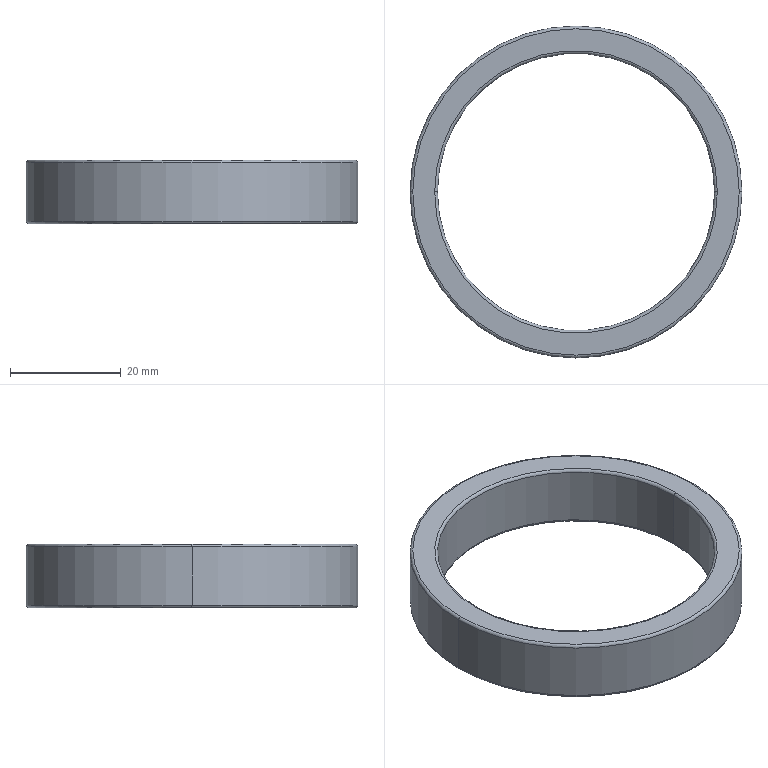Part | STEP file | 10-06 shaft shoulder | 1 solid | 14 faces | box 60 x 60 x 11.5 mm | volume 9808 mm3 | torus 8 | cylinder 4 | plane 2 | commonest cylinder face diameters 50.1 x2 60 x2
STEP:
#1=CARTESIAN_POINT('',(-30.,0.,5.25));
#2=VERTEX_POINT('',#1);
#3=CARTESIAN_POINT('',(30.,0.,5.25));
#4=VERTEX_POINT('',#3);
#5=CARTESIAN_POINT('',(0.,0.,5.25));
#6=DIRECTION('',(0.,0.,-1.));
#7=DIRECTION('',(1.,0.,0.));
#8=AXIS2_PLACEMENT_3D('',#5,#6,#7);
#9=CIRCLE('',#8,30.);
#10=EDGE_CURVE('',#2,#4,#9,.T.);
#11=ORIENTED_EDGE('',*,*,#10,.F.);
#12=CARTESIAN_POINT('',(-29.5,0.,5.75));
#13=VERTEX_POINT('',#12);
#14=CARTESIAN_POINT('',(-29.5,0.,5.25));
#15=DIRECTION('',(0.,1.,0.));
#16=DIRECTION('',(-1.,0.,0.));
#17=AXIS2_PLACEMENT_3D('',#14,#15,#16);
#18=CIRCLE('',#17,0.5);
#19=EDGE_CURVE('',#2,#13,#18,.T.);
#20=ORIENTED_EDGE('',*,*,#19,.T.);
#21=CARTESIAN_POINT('',(29.5,0.,5.75));
#22=VERTEX_POINT('',#21);
#23=CARTESIAN_POINT('',(0.,0.,5.75));
#24=DIRECTION('',(0.,0.,1.));
#25=DIRECTION('',(1.,0.,0.));
#26=AXIS2_PLACEMENT_3D('',#23,#24,#25);
#27=CIRCLE('',#26,29.5);
#28=EDGE_CURVE('',#22,#13,#27,.T.);
#29=ORIENTED_EDGE('',*,*,#28,.F.);
#30=CARTESIAN_POINT('',(29.5,0.,5.25));
#31=DIRECTION('',(0.,-1.,0.));
#32=DIRECTION('',(0.,0.,-1.));
#33=AXIS2_PLACEMENT_3D('',#30,#31,#32);
#34=CIRCLE('',#33,0.5);
#35=EDGE_CURVE('',#4,#22,#34,.T.);
#36=ORIENTED_EDGE('',*,*,#35,.F.);
#37=EDGE_LOOP('',(#11,#20,#29,#36));
#38=FACE_OUTER_BOUND('',#37,.T.);
#39=CARTESIAN_POINT('',(0.,0.,5.25));
#40=DIRECTION('',(0.,0.,1.));
#41=DIRECTION('',(1.,0.,0.));
#42=AXIS2_PLACEMENT_3D('',#39,#40,#41);
#43=TOROIDAL_SURFACE('',#42,29.5,0.5);
#44=ADVANCED_FACE('',(#38),#43,.T.);
#45=CARTESIAN_POINT('',(-29.5,0.,-5.75));
#46=VERTEX_POINT('',#45);
#47=CARTESIAN_POINT('',(29.5,0.,-5.75));
#48=VERTEX_POINT('',#47);
#49=CARTESIAN_POINT('',(0.,0.,-5.75));
#50=DIRECTION('',(0.,0.,-1.));
#51=DIRECTION('',(1.,0.,0.));
#52=AXIS2_PLACEMENT_3D('',#49,#50,#51);
#53=CIRCLE('',#52,29.5);
#54=EDGE_CURVE('',#46,#48,#53,.T.);
#55=ORIENTED_EDGE('',*,*,#54,.F.);
#56=CARTESIAN_POINT('',(-30.,0.,-5.25));
#57=VERTEX_POINT('',#56);
#58=CARTESIAN_POINT('',(-29.5,0.,-5.25));
#59=DIRECTION('',(0.,1.,0.));
#60=DIRECTION('',(-1.,0.,0.));
#61=AXIS2_PLACEMENT_3D('',#58,#59,#60);
#62=CIRCLE('',#61,0.5);
#63=EDGE_CURVE('',#46,#57,#62,.T.);
#64=ORIENTED_EDGE('',*,*,#63,.T.);
#65=CARTESIAN_POINT('',(30.,0.,-5.25));
#66=VERTEX_POINT('',#65);
#67=CARTESIAN_POINT('',(0.,0.,-5.25));
#68=DIRECTION('',(0.,0.,1.));
#69=DIRECTION('',(1.,0.,0.));
#70=AXIS2_PLACEMENT_3D('',#67,#68,#69);
#71=CIRCLE('',#70,30.);
#72=EDGE_CURVE('',#66,#57,#71,.T.);
#73=ORIENTED_EDGE('',*,*,#72,.F.);
#74=CARTESIAN_POINT('',(29.5,0.,-5.25));
#75=DIRECTION('',(0.,-1.,0.));
#76=DIRECTION('',(0.,0.,-1.));
#77=AXIS2_PLACEMENT_3D('',#74,#75,#76);
#78=CIRCLE('',#77,0.5);
#79=EDGE_CURVE('',#48,#66,#78,.T.);
#80=ORIENTED_EDGE('',*,*,#79,.F.);
#81=EDGE_LOOP('',(#55,#64,#73,#80));
#82=FACE_OUTER_BOUND('',#81,.T.);
#83=CARTESIAN_POINT('',(0.,0.,-5.25));
#84=DIRECTION('',(0.,0.,1.));
#85=DIRECTION('',(1.,0.,0.));
#86=AXIS2_PLACEMENT_3D('',#83,#84,#85);
#87=TOROIDAL_SURFACE('',#86,29.5,0.5);
#88=ADVANCED_FACE('',(#82),#87,.T.);
#89=CARTESIAN_POINT('',(-25.05,0.,-5.25));
#90=VERTEX_POINT('',#89);
#91=CARTESIAN_POINT('',(25.05,0.,-5.25));
#92=VERTEX_POINT('',#91);
#93=CARTESIAN_POINT('',(0.,0.,-5.25));
#94=DIRECTION('',(0.,0.,-1.));
#95=DIRECTION('',(1.,0.,0.));
#96=AXIS2_PLACEMENT_3D('',#93,#94,#95);
#97=CIRCLE('',#96,25.05);
#98=EDGE_CURVE('',#90,#92,#97,.T.);
#99=ORIENTED_EDGE('',*,*,#98,.F.);
#100=CARTESIAN_POINT('',(-25.55,0.,-5.75));
#101=VERTEX_POINT('',#100);
#102=CARTESIAN_POINT('',(-25.55,0.,-5.25));
#103=DIRECTION('',(0.,1.,0.));
#104=DIRECTION('',(-1.,0.,0.));
#105=AXIS2_PLACEMENT_3D('',#102,#103,#104);
#106=CIRCLE('',#105,0.5);
#107=EDGE_CURVE('',#90,#101,#106,.T.);
#108=ORIENTED_EDGE('',*,*,#107,.T.);
#109=CARTESIAN_POINT('',(25.55,0.,-5.75));
#110=VERTEX_POINT('',#109);
#111=CARTESIAN_POINT('',(0.,0.,-5.75));
#112=DIRECTION('',(0.,0.,1.));
#113=DIRECTION('',(1.,0.,0.));
#114=AXIS2_PLACEMENT_3D('',#111,#112,#113);
#115=CIRCLE('',#114,25.55);
#116=EDGE_CURVE('',#110,#101,#115,.T.);
#117=ORIENTED_EDGE('',*,*,#116,.F.);
#118=CARTESIAN_POINT('',(25.55,0.,-5.25));
#119=DIRECTION('',(0.,-1.,0.));
#120=DIRECTION('',(0.,0.,-1.));
#121=AXIS2_PLACEMENT_3D('',#118,#119,#120);
#122=CIRCLE('',#121,0.5);
#123=EDGE_CURVE('',#92,#110,#122,.T.);
#124=ORIENTED_EDGE('',*,*,#123,.F.);
#125=EDGE_LOOP('',(#99,#108,#117,#124));
#126=FACE_OUTER_BOUND('',#125,.T.);
#127=CARTESIAN_POINT('',(0.,0.,-5.25));
#128=DIRECTION('',(0.,0.,1.));
#129=DIRECTION('',(1.,0.,0.));
#130=AXIS2_PLACEMENT_3D('',#127,#128,#129);
#131=TOROIDAL_SURFACE('',#130,25.55,0.5);
#132=ADVANCED_FACE('',(#126),#131,.T.);
#133=CARTESIAN_POINT('',(-25.55,0.,5.75));
#134=VERTEX_POINT('',#133);
#135=CARTESIAN_POINT('',(25.55,0.,5.75));
#136=VERTEX_POINT('',#135);
#137=CARTESIAN_POINT('',(0.,0.,5.75));
#138=DIRECTION('',(0.,0.,-1.));
#139=DIRECTION('',(1.,0.,0.));
#140=AXIS2_PLACEMENT_3D('',#137,#138,#139);
#141=CIRCLE('',#140,25.55);
#142=EDGE_CURVE('',#134,#136,#141,.T.);
#143=ORIENTED_EDGE('',*,*,#142,.F.);
#144=CARTESIAN_POINT('',(-25.05,0.,5.25));
#145=VERTEX_POINT('',#144);
#146=CARTESIAN_POINT('',(-25.55,0.,5.25));
#147=DIRECTION('',(0.,1.,0.));
#148=DIRECTION('',(-1.,0.,0.));
#149=AXIS2_PLACEMENT_3D('',#146,#147,#148);
#150=CIRCLE('',#149,0.5);
#151=EDGE_CURVE('',#134,#145,#150,.T.);
#152=ORIENTED_EDGE('',*,*,#151,.T.);
#153=CARTESIAN_POINT('',(25.05,0.,5.25));
#154=VERTEX_POINT('',#153);
#155=CARTESIAN_POINT('',(0.,0.,5.25));
#156=DIRECTION('',(0.,0.,1.));
#157=DIRECTION('',(1.,0.,0.));
#158=AXIS2_PLACEMENT_3D('',#155,#156,#157);
#159=CIRCLE('',#158,25.05);
#160=EDGE_CURVE('',#154,#145,#159,.T.);
#161=ORIENTED_EDGE('',*,*,#160,.F.);
#162=CARTESIAN_POINT('',(25.55,0.,5.25));
#163=DIRECTION('',(0.,-1.,0.));
#164=DIRECTION('',(0.,0.,-1.));
#165=AXIS2_PLACEMENT_3D('',#162,#163,#164);
#166=CIRCLE('',#165,0.5);
#167=EDGE_CURVE('',#136,#154,#166,.T.);
#168=ORIENTED_EDGE('',*,*,#167,.F.);
#169=EDGE_LOOP('',(#143,#152,#161,#168));
#170=FACE_OUTER_BOUND('',#169,.T.);
#171=CARTESIAN_POINT('',(0.,0.,5.25));
#172=DIRECTION('',(0.,0.,1.));
#173=DIRECTION('',(1.,0.,0.));
#174=AXIS2_PLACEMENT_3D('',#171,#172,#173);
#175=TOROIDAL_SURFACE('',#174,25.55,0.5);
#176=ADVANCED_FACE('',(#170),#175,.T.);
#177=CARTESIAN_POINT('',(0.,0.,5.25));
#178=DIRECTION('',(0.,0.,1.));
#179=DIRECTION('',(1.,0.,0.));
#180=AXIS2_PLACEMENT_3D('',#177,#178,#179);
#181=CIRCLE('',#180,25.05);
#182=EDGE_CURVE('',#145,#154,#181,.T.);
#183=ORIENTED_EDGE('',*,*,#182,.T.);
#184=CARTESIAN_POINT('',(25.05,0.,5.75));
#185=DIRECTION('',(0.,0.,-1.));
#186=VECTOR('',#185,1000.);
#187=LINE('',#184,#186);
#188=EDGE_CURVE('',#154,#92,#187,.T.);
#189=ORIENTED_EDGE('',*,*,#188,.T.);
#190=CARTESIAN_POINT('',(0.,0.,-5.25));
#191=DIRECTION('',(0.,0.,-1.));
#192=DIRECTION('',(1.,0.,0.));
#193=AXIS2_PLACEMENT_3D('',#190,#191,#192);
#194=CIRCLE('',#193,25.05);
#195=EDGE_CURVE('',#92,#90,#194,.T.);
#196=ORIENTED_EDGE('',*,*,#195,.T.);
#197=CARTESIAN_POINT('',(-25.05,0.,5.75));
#198=DIRECTION('',(0.,0.,-1.));
#199=VECTOR('',#198,1000.);
#200=LINE('',#197,#199);
#201=EDGE_CURVE('',#145,#90,#200,.T.);
#202=ORIENTED_EDGE('',*,*,#201,.F.);
#203=EDGE_LOOP('',(#183,#189,#196,#202));
#204=FACE_OUTER_BOUND('',#203,.T.);
#205=CARTESIAN_POINT('',(0.,0.,5.75));
#206=DIRECTION('',(0.,0.,-1.));
#207=DIRECTION('',(-1.,0.,0.));
#208=AXIS2_PLACEMENT_3D('',#205,#206,#207);
#209=CYLINDRICAL_SURFACE('',#208,25.05);
#210=ADVANCED_FACE('',(#204),#209,.F.);
#211=ORIENTED_EDGE('',*,*,#10,.T.);
#212=CARTESIAN_POINT('',(30.,0.,5.75));
#213=DIRECTION('',(0.,0.,-1.));
#214=VECTOR('',#213,1000.);
#215=LINE('',#212,#214);
#216=EDGE_CURVE('',#4,#66,#215,.T.);
#217=ORIENTED_EDGE('',*,*,#216,.T.);
#218=ORIENTED_EDGE('',*,*,#72,.T.);
#219=CARTESIAN_POINT('',(-30.,0.,5.75));
#220=DIRECTION('',(0.,0.,-1.));
#221=VECTOR('',#220,1000.);
#222=LINE('',#219,#221);
#223=EDGE_CURVE('',#2,#57,#222,.T.);
#224=ORIENTED_EDGE('',*,*,#223,.F.);
#225=EDGE_LOOP('',(#211,#217,#218,#224));
#226=FACE_OUTER_BOUND('',#225,.T.);
#227=CARTESIAN_POINT('',(0.,0.,5.75));
#228=DIRECTION('',(0.,0.,-1.));
#229=DIRECTION('',(-1.,0.,0.));
#230=AXIS2_PLACEMENT_3D('',#227,#228,#229);
#231=CYLINDRICAL_SURFACE('',#230,30.);
#232=ADVANCED_FACE('',(#226),#231,.T.);
#233=CARTESIAN_POINT('',(0.,0.,5.75));
#234=DIRECTION('',(0.,0.,-1.));
#235=DIRECTION('',(1.,0.,0.));
#236=AXIS2_PLACEMENT_3D('',#233,#234,#235);
#237=CIRCLE('',#236,25.55);
#238=EDGE_CURVE('',#136,#134,#237,.T.);
#239=ORIENTED_EDGE('',*,*,#238,.T.);
#240=ORIENTED_EDGE('',*,*,#142,.T.);
#241=EDGE_LOOP('',(#239,#240));
#242=FACE_BOUND('',#241,.T.);
#243=ORIENTED_EDGE('',*,*,#28,.T.);
#244=CARTESIAN_POINT('',(0.,0.,5.75));
#245=DIRECTION('',(0.,0.,1.));
#246=DIRECTION('',(1.,0.,0.));
#247=AXIS2_PLACEMENT_3D('',#244,#245,#246);
#248=CIRCLE('',#247,29.5);
#249=EDGE_CURVE('',#13,#22,#248,.T.);
#250=ORIENTED_EDGE('',*,*,#249,.T.);
#251=EDGE_LOOP('',(#243,#250));
#252=FACE_OUTER_BOUND('',#251,.T.);
#253=CARTESIAN_POINT('',(0.,0.,5.75));
#254=DIRECTION('',(0.,0.,1.));
#255=DIRECTION('',(1.,0.,0.));
#256=AXIS2_PLACEMENT_3D('',#253,#254,#255);
#257=PLANE('',#256);
#258=ADVANCED_FACE('',(#242,#252),#257,.T.);
#259=ORIENTED_EDGE('',*,*,#116,.T.);
#260=CARTESIAN_POINT('',(0.,0.,-5.75));
#261=DIRECTION('',(0.,0.,1.));
#262=DIRECTION('',(1.,0.,0.));
#263=AXIS2_PLACEMENT_3D('',#260,#261,#262);
#264=CIRCLE('',#263,25.55);
#265=EDGE_CURVE('',#101,#110,#264,.T.);
#266=ORIENTED_EDGE('',*,*,#265,.T.);
#267=EDGE_LOOP('',(#259,#266));
#268=FACE_BOUND('',#267,.T.);
#269=CARTESIAN_POINT('',(0.,0.,-5.75));
#270=DIRECTION('',(0.,0.,-1.));
#271=DIRECTION('',(1.,0.,0.));
#272=AXIS2_PLACEMENT_3D('',#269,#270,#271);
#273=CIRCLE('',#272,29.5);
#274=EDGE_CURVE('',#48,#46,#273,.T.);
#275=ORIENTED_EDGE('',*,*,#274,.T.);
#276=ORIENTED_EDGE('',*,*,#54,.T.);
#277=EDGE_LOOP('',(#275,#276));
#278=FACE_OUTER_BOUND('',#277,.T.);
#279=CARTESIAN_POINT('',(0.,0.,-5.75));
#280=DIRECTION('',(0.,0.,1.));
#281=DIRECTION('',(1.,0.,0.));
#282=AXIS2_PLACEMENT_3D('',#279,#280,#281);
#283=PLANE('',#282);
#284=ADVANCED_FACE('',(#268,#278),#283,.F.);
#285=ORIENTED_EDGE('',*,*,#216,.F.);
#286=CARTESIAN_POINT('',(0.,0.,5.25));
#287=DIRECTION('',(0.,0.,-1.));
#288=DIRECTION('',(1.,0.,0.));
#289=AXIS2_PLACEMENT_3D('',#286,#287,#288);
#290=CIRCLE('',#289,30.);
#291=EDGE_CURVE('',#4,#2,#290,.T.);
#292=ORIENTED_EDGE('',*,*,#291,.T.);
#293=ORIENTED_EDGE('',*,*,#223,.T.);
#294=CARTESIAN_POINT('',(0.,0.,-5.25));
#295=DIRECTION('',(0.,0.,1.));
#296=DIRECTION('',(1.,0.,0.));
#297=AXIS2_PLACEMENT_3D('',#294,#295,#296);
#298=CIRCLE('',#297,30.);
#299=EDGE_CURVE('',#57,#66,#298,.T.);
#300=ORIENTED_EDGE('',*,*,#299,.T.);
#301=EDGE_LOOP('',(#285,#292,#293,#300));
#302=FACE_OUTER_BOUND('',#301,.T.);
#303=CARTESIAN_POINT('',(0.,0.,5.75));
#304=DIRECTION('',(0.,0.,-1.));
#305=DIRECTION('',(-1.,0.,0.));
#306=AXIS2_PLACEMENT_3D('',#303,#304,#305);
#307=CYLINDRICAL_SURFACE('',#306,30.);
#308=ADVANCED_FACE('',(#302),#307,.T.);
#309=ORIENTED_EDGE('',*,*,#188,.F.);
#310=ORIENTED_EDGE('',*,*,#160,.T.);
#311=ORIENTED_EDGE('',*,*,#201,.T.);
#312=ORIENTED_EDGE('',*,*,#98,.T.);
#313=EDGE_LOOP('',(#309,#310,#311,#312));
#314=FACE_OUTER_BOUND('',#313,.T.);
#315=CARTESIAN_POINT('',(0.,0.,5.75));
#316=DIRECTION('',(0.,0.,-1.));
#317=DIRECTION('',(-1.,0.,0.));
#318=AXIS2_PLACEMENT_3D('',#315,#316,#317);
#319=CYLINDRICAL_SURFACE('',#318,25.05);
#320=ADVANCED_FACE('',(#314),#319,.F.);
#321=ORIENTED_EDGE('',*,*,#151,.F.);
#322=ORIENTED_EDGE('',*,*,#238,.F.);
#323=ORIENTED_EDGE('',*,*,#167,.T.);
#324=ORIENTED_EDGE('',*,*,#182,.F.);
#325=EDGE_LOOP('',(#321,#322,#323,#324));
#326=FACE_OUTER_BOUND('',#325,.T.);
#327=CARTESIAN_POINT('',(0.,0.,5.25));
#328=DIRECTION('',(0.,0.,1.));
#329=DIRECTION('',(1.,0.,0.));
#330=AXIS2_PLACEMENT_3D('',#327,#328,#329);
#331=TOROIDAL_SURFACE('',#330,25.55,0.5);
#332=ADVANCED_FACE('',(#326),#331,.T.);
#333=ORIENTED_EDGE('',*,*,#107,.F.);
#334=ORIENTED_EDGE('',*,*,#195,.F.);
#335=ORIENTED_EDGE('',*,*,#123,.T.);
#336=ORIENTED_EDGE('',*,*,#265,.F.);
#337=EDGE_LOOP('',(#333,#334,#335,#336));
#338=FACE_OUTER_BOUND('',#337,.T.);
#339=CARTESIAN_POINT('',(0.,0.,-5.25));
#340=DIRECTION('',(0.,0.,1.));
#341=DIRECTION('',(1.,0.,0.));
#342=AXIS2_PLACEMENT_3D('',#339,#340,#341);
#343=TOROIDAL_SURFACE('',#342,25.55,0.5);
#344=ADVANCED_FACE('',(#338),#343,.T.);
#345=ORIENTED_EDGE('',*,*,#63,.F.);
#346=ORIENTED_EDGE('',*,*,#274,.F.);
#347=ORIENTED_EDGE('',*,*,#79,.T.);
#348=ORIENTED_EDGE('',*,*,#299,.F.);
#349=EDGE_LOOP('',(#345,#346,#347,#348));
#350=FACE_OUTER_BOUND('',#349,.T.);
#351=CARTESIAN_POINT('',(0.,0.,-5.25));
#352=DIRECTION('',(0.,0.,1.));
#353=DIRECTION('',(1.,0.,0.));
#354=AXIS2_PLACEMENT_3D('',#351,#352,#353);
#355=TOROIDAL_SURFACE('',#354,29.5,0.5);
#356=ADVANCED_FACE('',(#350),#355,.T.);
#357=ORIENTED_EDGE('',*,*,#19,.F.);
#358=ORIENTED_EDGE('',*,*,#291,.F.);
#359=ORIENTED_EDGE('',*,*,#35,.T.);
#360=ORIENTED_EDGE('',*,*,#249,.F.);
#361=EDGE_LOOP('',(#357,#358,#359,#360));
#362=FACE_OUTER_BOUND('',#361,.T.);
#363=CARTESIAN_POINT('',(0.,0.,5.25));
#364=DIRECTION('',(0.,0.,1.));
#365=DIRECTION('',(1.,0.,0.));
#366=AXIS2_PLACEMENT_3D('',#363,#364,#365);
#367=TOROIDAL_SURFACE('',#366,29.5,0.5);
#368=ADVANCED_FACE('',(#362),#367,.T.);
#369=CLOSED_SHELL('',(#44,#88,#132,#176,#210,#232,#258,#284,#308,#320,#332,#344,#356,#368));
#370=MANIFOLD_SOLID_BREP('',#369);
#371=CARTESIAN_POINT('',(0.,0.,0.));
#372=DIRECTION('',(0.,0.,1.));
#373=DIRECTION('',(1.,0.,0.));
#374=AXIS2_PLACEMENT_3D('',#371,#372,#373);
#375=(LENGTH_UNIT()NAMED_UNIT(*)SI_UNIT(.MILLI.,.METRE.));
#376=UNCERTAINTY_MEASURE_WITH_UNIT(LENGTH_MEASURE(0.00001),#375,'','');
#377=(NAMED_UNIT(*)PLANE_ANGLE_UNIT()SI_UNIT($,.RADIAN.));
#378=(NAMED_UNIT(*)SI_UNIT($,.STERADIAN.)SOLID_ANGLE_UNIT());
#379=(GEOMETRIC_REPRESENTATION_CONTEXT(3)GLOBAL_UNCERTAINTY_ASSIGNED_CONTEXT((#376))GLOBAL_UNIT_ASSIGNED_CONTEXT((#375,#377,#378))REPRESENTATION_CONTEXT('',''));
#380=ADVANCED_BREP_SHAPE_REPRESENTATION('',(#370,#374),#379);